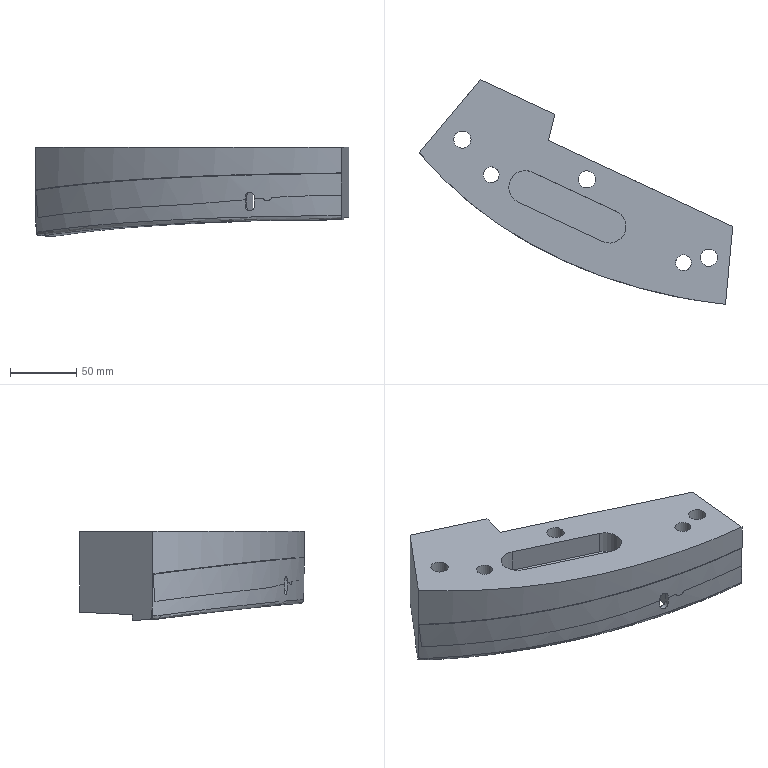Part | NX | features solid 2 | 1 solid | 69 faces | box 236.514 x 169.502 x 67.201 mm | volume 879124 mm3 | plane 26 | spline 21 | cylinder 19 | sphere 2 | cone 1 | commonest cylinder face diameters 10 x5 13 x3 20 x3 7.1 x2 12 x2 25 x2